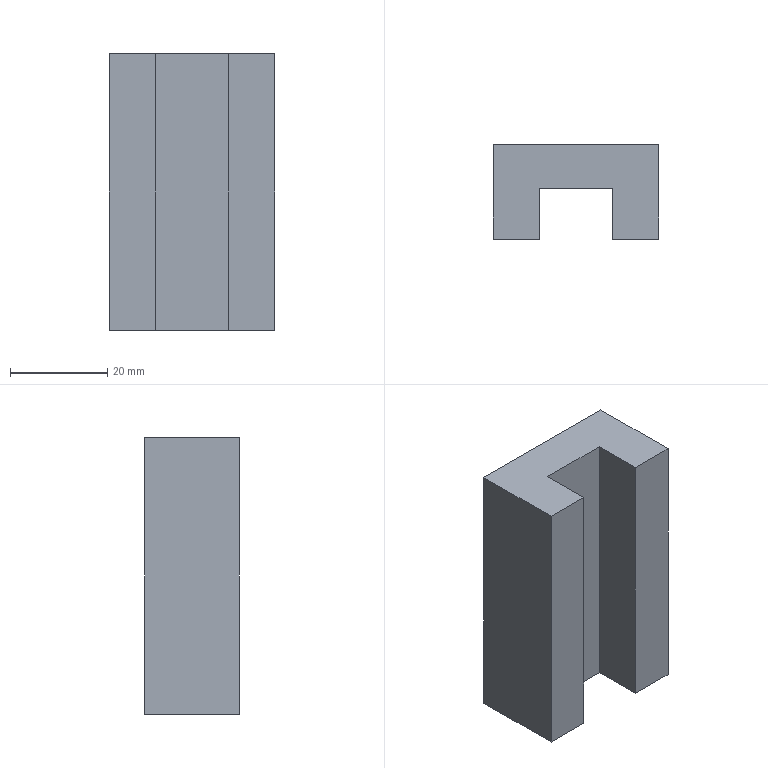Part | SolidWorks | features ICE 2, Extrusion 1 | 1 solid | 22 faces | box 34 x 19.5 x 56.8 mm | volume 28468 mm3 | plane 14 | cylinder 8 | commonest cylinder face diameters 3.6 x8
STEP:
#1=CARTESIAN_POINT('',(-13.,3.75,11.2));
#2=VERTEX_POINT('',#1);
#3=CARTESIAN_POINT('',(-13.,3.75,14.8));
#4=VERTEX_POINT('',#3);
#5=CARTESIAN_POINT('',(-13.,3.75,13.));
#6=DIRECTION('',(0.,1.,0.));
#7=DIRECTION('',(0.,0.,-1.));
#8=AXIS2_PLACEMENT_3D('',#5,#6,#7);
#9=CIRCLE('',#8,1.8);
#10=EDGE_CURVE('',#2,#4,#9,.T.);
#11=ORIENTED_EDGE('',*,*,#10,.F.);
#12=CARTESIAN_POINT('',(-13.,9.75,11.2));
#13=VERTEX_POINT('',#12);
#14=CARTESIAN_POINT('',(-13.,3.75,11.2));
#15=DIRECTION('',(0.,1.,0.));
#16=VECTOR('',#15,1000.);
#17=LINE('',#14,#16);
#18=EDGE_CURVE('',#2,#13,#17,.T.);
#19=ORIENTED_EDGE('',*,*,#18,.T.);
#20=CARTESIAN_POINT('',(-13.,9.75,14.8));
#21=VERTEX_POINT('',#20);
#22=CARTESIAN_POINT('',(-13.,9.75,13.));
#23=DIRECTION('',(0.,1.,0.));
#24=DIRECTION('',(0.,0.,-1.));
#25=AXIS2_PLACEMENT_3D('',#22,#23,#24);
#26=CIRCLE('',#25,1.8);
#27=EDGE_CURVE('',#13,#21,#26,.T.);
#28=ORIENTED_EDGE('',*,*,#27,.T.);
#29=CARTESIAN_POINT('',(-13.,3.75,14.8));
#30=DIRECTION('',(0.,1.,0.));
#31=VECTOR('',#30,1000.);
#32=LINE('',#29,#31);
#33=EDGE_CURVE('',#4,#21,#32,.T.);
#34=ORIENTED_EDGE('',*,*,#33,.F.);
#35=EDGE_LOOP('',(#11,#19,#28,#34));
#36=FACE_OUTER_BOUND('',#35,.T.);
#37=CARTESIAN_POINT('',(-13.,3.75,13.));
#38=DIRECTION('',(0.,1.,0.));
#39=DIRECTION('',(0.,0.,1.));
#40=AXIS2_PLACEMENT_3D('',#37,#38,#39);
#41=CYLINDRICAL_SURFACE('',#40,1.8);
#42=ADVANCED_FACE('',(#36),#41,.F.);
#43=CARTESIAN_POINT('',(13.,3.75,11.2));
#44=VERTEX_POINT('',#43);
#45=CARTESIAN_POINT('',(13.,3.75,14.8));
#46=VERTEX_POINT('',#45);
#47=CARTESIAN_POINT('',(13.,3.75,13.));
#48=DIRECTION('',(0.,1.,0.));
#49=DIRECTION('',(0.,0.,1.));
#50=AXIS2_PLACEMENT_3D('',#47,#48,#49);
#51=CIRCLE('',#50,1.8);
#52=EDGE_CURVE('',#44,#46,#51,.T.);
#53=ORIENTED_EDGE('',*,*,#52,.F.);
#54=CARTESIAN_POINT('',(13.,9.75,11.2));
#55=VERTEX_POINT('',#54);
#56=CARTESIAN_POINT('',(13.,3.75,11.2));
#57=DIRECTION('',(0.,1.,0.));
#58=VECTOR('',#57,1000.);
#59=LINE('',#56,#58);
#60=EDGE_CURVE('',#44,#55,#59,.T.);
#61=ORIENTED_EDGE('',*,*,#60,.T.);
#62=CARTESIAN_POINT('',(13.,9.75,14.8));
#63=VERTEX_POINT('',#62);
#64=CARTESIAN_POINT('',(13.,9.75,13.));
#65=DIRECTION('',(0.,1.,0.));
#66=DIRECTION('',(0.,0.,1.));
#67=AXIS2_PLACEMENT_3D('',#64,#65,#66);
#68=CIRCLE('',#67,1.8);
#69=EDGE_CURVE('',#55,#63,#68,.T.);
#70=ORIENTED_EDGE('',*,*,#69,.T.);
#71=CARTESIAN_POINT('',(13.,3.75,14.8));
#72=DIRECTION('',(0.,1.,0.));
#73=VECTOR('',#72,1000.);
#74=LINE('',#71,#73);
#75=EDGE_CURVE('',#46,#63,#74,.T.);
#76=ORIENTED_EDGE('',*,*,#75,.F.);
#77=EDGE_LOOP('',(#53,#61,#70,#76));
#78=FACE_OUTER_BOUND('',#77,.T.);
#79=CARTESIAN_POINT('',(13.,3.75,13.));
#80=DIRECTION('',(0.,1.,0.));
#81=DIRECTION('',(0.,0.,1.));
#82=AXIS2_PLACEMENT_3D('',#79,#80,#81);
#83=CYLINDRICAL_SURFACE('',#82,1.8);
#84=ADVANCED_FACE('',(#78),#83,.F.);
#85=CARTESIAN_POINT('',(13.,3.75,-14.8));
#86=VERTEX_POINT('',#85);
#87=CARTESIAN_POINT('',(13.,3.75,-11.2));
#88=VERTEX_POINT('',#87);
#89=CARTESIAN_POINT('',(13.,3.75,-13.));
#90=DIRECTION('',(0.,1.,0.));
#91=DIRECTION('',(0.,0.,-1.));
#92=AXIS2_PLACEMENT_3D('',#89,#90,#91);
#93=CIRCLE('',#92,1.8);
#94=EDGE_CURVE('',#86,#88,#93,.T.);
#95=ORIENTED_EDGE('',*,*,#94,.F.);
#96=CARTESIAN_POINT('',(13.,9.75,-14.8));
#97=VERTEX_POINT('',#96);
#98=CARTESIAN_POINT('',(13.,3.75,-14.8));
#99=DIRECTION('',(0.,1.,0.));
#100=VECTOR('',#99,1000.);
#101=LINE('',#98,#100);
#102=EDGE_CURVE('',#86,#97,#101,.T.);
#103=ORIENTED_EDGE('',*,*,#102,.T.);
#104=CARTESIAN_POINT('',(13.,9.75,-11.2));
#105=VERTEX_POINT('',#104);
#106=CARTESIAN_POINT('',(13.,9.75,-13.));
#107=DIRECTION('',(0.,1.,0.));
#108=DIRECTION('',(0.,0.,-1.));
#109=AXIS2_PLACEMENT_3D('',#106,#107,#108);
#110=CIRCLE('',#109,1.8);
#111=EDGE_CURVE('',#97,#105,#110,.T.);
#112=ORIENTED_EDGE('',*,*,#111,.T.);
#113=CARTESIAN_POINT('',(13.,3.75,-11.2));
#114=DIRECTION('',(0.,1.,0.));
#115=VECTOR('',#114,1000.);
#116=LINE('',#113,#115);
#117=EDGE_CURVE('',#88,#105,#116,.T.);
#118=ORIENTED_EDGE('',*,*,#117,.F.);
#119=EDGE_LOOP('',(#95,#103,#112,#118));
#120=FACE_OUTER_BOUND('',#119,.T.);
#121=CARTESIAN_POINT('',(13.,3.75,-13.));
#122=DIRECTION('',(0.,1.,0.));
#123=DIRECTION('',(0.,0.,1.));
#124=AXIS2_PLACEMENT_3D('',#121,#122,#123);
#125=CYLINDRICAL_SURFACE('',#124,1.8);
#126=ADVANCED_FACE('',(#120),#125,.F.);
#127=CARTESIAN_POINT('',(-13.,3.75,-14.8));
#128=VERTEX_POINT('',#127);
#129=CARTESIAN_POINT('',(-13.,3.75,-11.2));
#130=VERTEX_POINT('',#129);
#131=CARTESIAN_POINT('',(-13.,3.75,-13.));
#132=DIRECTION('',(0.,1.,0.));
#133=DIRECTION('',(0.,0.,1.));
#134=AXIS2_PLACEMENT_3D('',#131,#132,#133);
#135=CIRCLE('',#134,1.8);
#136=EDGE_CURVE('',#128,#130,#135,.T.);
#137=ORIENTED_EDGE('',*,*,#136,.F.);
#138=CARTESIAN_POINT('',(-13.,9.75,-14.8));
#139=VERTEX_POINT('',#138);
#140=CARTESIAN_POINT('',(-13.,3.75,-14.8));
#141=DIRECTION('',(0.,1.,0.));
#142=VECTOR('',#141,1000.);
#143=LINE('',#140,#142);
#144=EDGE_CURVE('',#128,#139,#143,.T.);
#145=ORIENTED_EDGE('',*,*,#144,.T.);
#146=CARTESIAN_POINT('',(-13.,9.75,-11.2));
#147=VERTEX_POINT('',#146);
#148=CARTESIAN_POINT('',(-13.,9.75,-13.));
#149=DIRECTION('',(0.,1.,0.));
#150=DIRECTION('',(0.,0.,1.));
#151=AXIS2_PLACEMENT_3D('',#148,#149,#150);
#152=CIRCLE('',#151,1.8);
#153=EDGE_CURVE('',#139,#147,#152,.T.);
#154=ORIENTED_EDGE('',*,*,#153,.T.);
#155=CARTESIAN_POINT('',(-13.,3.75,-11.2));
#156=DIRECTION('',(0.,1.,0.));
#157=VECTOR('',#156,1000.);
#158=LINE('',#155,#157);
#159=EDGE_CURVE('',#130,#147,#158,.T.);
#160=ORIENTED_EDGE('',*,*,#159,.F.);
#161=EDGE_LOOP('',(#137,#145,#154,#160));
#162=FACE_OUTER_BOUND('',#161,.T.);
#163=CARTESIAN_POINT('',(-13.,3.75,-13.));
#164=DIRECTION('',(0.,1.,0.));
#165=DIRECTION('',(0.,0.,1.));
#166=AXIS2_PLACEMENT_3D('',#163,#164,#165);
#167=CYLINDRICAL_SURFACE('',#166,1.8);
#168=ADVANCED_FACE('',(#162),#167,.F.);
#169=CARTESIAN_POINT('',(7.5,-9.75,28.4));
#170=VERTEX_POINT('',#169);
#171=CARTESIAN_POINT('',(17.,-9.75,28.4));
#172=VERTEX_POINT('',#171);
#173=CARTESIAN_POINT('',(-17.,-9.75,28.4));
#174=DIRECTION('',(1.,0.,0.));
#175=VECTOR('',#174,1000.);
#176=LINE('',#173,#175);
#177=EDGE_CURVE('',#170,#172,#176,.T.);
#178=ORIENTED_EDGE('',*,*,#177,.F.);
#179=CARTESIAN_POINT('',(7.5,-9.75,-28.4));
#180=VERTEX_POINT('',#179);
#181=CARTESIAN_POINT('',(7.5,-9.75,-28.4));
#182=DIRECTION('',(0.,0.,1.));
#183=VECTOR('',#182,1000.);
#184=LINE('',#181,#183);
#185=EDGE_CURVE('',#180,#170,#184,.T.);
#186=ORIENTED_EDGE('',*,*,#185,.F.);
#187=CARTESIAN_POINT('',(17.,-9.75,-28.4));
#188=VERTEX_POINT('',#187);
#189=CARTESIAN_POINT('',(-17.,-9.75,-28.4));
#190=DIRECTION('',(1.,0.,0.));
#191=VECTOR('',#190,1000.);
#192=LINE('',#189,#191);
#193=EDGE_CURVE('',#180,#188,#192,.T.);
#194=ORIENTED_EDGE('',*,*,#193,.T.);
#195=CARTESIAN_POINT('',(17.,-9.75,28.4));
#196=DIRECTION('',(0.,0.,-1.));
#197=VECTOR('',#196,1000.);
#198=LINE('',#195,#197);
#199=EDGE_CURVE('',#172,#188,#198,.T.);
#200=ORIENTED_EDGE('',*,*,#199,.F.);
#201=EDGE_LOOP('',(#178,#186,#194,#200));
#202=FACE_OUTER_BOUND('',#201,.T.);
#203=CARTESIAN_POINT('',(-17.,-9.75,28.4));
#204=DIRECTION('',(0.,1.,0.));
#205=DIRECTION('',(0.,0.,1.));
#206=AXIS2_PLACEMENT_3D('',#203,#204,#205);
#207=PLANE('',#206);
#208=ADVANCED_FACE('',(#202),#207,.F.);
#209=CARTESIAN_POINT('',(17.,9.75,-28.4));
#210=VERTEX_POINT('',#209);
#211=CARTESIAN_POINT('',(17.,9.75,-28.4));
#212=DIRECTION('',(0.,1.,0.));
#213=VECTOR('',#212,1000.);
#214=LINE('',#211,#213);
#215=EDGE_CURVE('',#188,#210,#214,.T.);
#216=ORIENTED_EDGE('',*,*,#215,.T.);
#217=CARTESIAN_POINT('',(17.,9.75,28.4));
#218=VERTEX_POINT('',#217);
#219=CARTESIAN_POINT('',(17.,9.75,28.4));
#220=DIRECTION('',(0.,0.,-1.));
#221=VECTOR('',#220,1000.);
#222=LINE('',#219,#221);
#223=EDGE_CURVE('',#218,#210,#222,.T.);
#224=ORIENTED_EDGE('',*,*,#223,.F.);
#225=CARTESIAN_POINT('',(17.,9.75,28.4));
#226=DIRECTION('',(0.,1.,0.));
#227=VECTOR('',#226,1000.);
#228=LINE('',#225,#227);
#229=EDGE_CURVE('',#172,#218,#228,.T.);
#230=ORIENTED_EDGE('',*,*,#229,.F.);
#231=ORIENTED_EDGE('',*,*,#199,.T.);
#232=EDGE_LOOP('',(#216,#224,#230,#231));
#233=FACE_OUTER_BOUND('',#232,.T.);
#234=CARTESIAN_POINT('',(17.,9.75,28.4));
#235=DIRECTION('',(-1.,0.,0.));
#236=DIRECTION('',(0.,-1.,0.));
#237=AXIS2_PLACEMENT_3D('',#234,#235,#236);
#238=PLANE('',#237);
#239=ADVANCED_FACE('',(#233),#238,.F.);
#240=CARTESIAN_POINT('',(-13.,9.75,13.));
#241=DIRECTION('',(0.,1.,0.));
#242=DIRECTION('',(0.,0.,-1.));
#243=AXIS2_PLACEMENT_3D('',#240,#241,#242);
#244=CIRCLE('',#243,1.8);
#245=EDGE_CURVE('',#21,#13,#244,.T.);
#246=ORIENTED_EDGE('',*,*,#245,.F.);
#247=ORIENTED_EDGE('',*,*,#27,.F.);
#248=EDGE_LOOP('',(#246,#247));
#249=FACE_BOUND('',#248,.T.);
#250=CARTESIAN_POINT('',(13.,9.75,13.));
#251=DIRECTION('',(0.,1.,0.));
#252=DIRECTION('',(0.,0.,1.));
#253=AXIS2_PLACEMENT_3D('',#250,#251,#252);
#254=CIRCLE('',#253,1.8);
#255=EDGE_CURVE('',#63,#55,#254,.T.);
#256=ORIENTED_EDGE('',*,*,#255,.F.);
#257=ORIENTED_EDGE('',*,*,#69,.F.);
#258=EDGE_LOOP('',(#256,#257));
#259=FACE_BOUND('',#258,.T.);
#260=CARTESIAN_POINT('',(13.,9.75,-13.));
#261=DIRECTION('',(0.,1.,0.));
#262=DIRECTION('',(0.,0.,-1.));
#263=AXIS2_PLACEMENT_3D('',#260,#261,#262);
#264=CIRCLE('',#263,1.8);
#265=EDGE_CURVE('',#105,#97,#264,.T.);
#266=ORIENTED_EDGE('',*,*,#265,.F.);
#267=ORIENTED_EDGE('',*,*,#111,.F.);
#268=EDGE_LOOP('',(#266,#267));
#269=FACE_BOUND('',#268,.T.);
#270=CARTESIAN_POINT('',(-13.,9.75,-13.));
#271=DIRECTION('',(0.,1.,0.));
#272=DIRECTION('',(0.,0.,1.));
#273=AXIS2_PLACEMENT_3D('',#270,#271,#272);
#274=CIRCLE('',#273,1.8);
#275=EDGE_CURVE('',#147,#139,#274,.T.);
#276=ORIENTED_EDGE('',*,*,#275,.F.);
#277=ORIENTED_EDGE('',*,*,#153,.F.);
#278=EDGE_LOOP('',(#276,#277));
#279=FACE_BOUND('',#278,.T.);
#280=CARTESIAN_POINT('',(-17.,9.75,-28.4));
#281=VERTEX_POINT('',#280);
#282=CARTESIAN_POINT('',(-17.,9.75,-28.4));
#283=DIRECTION('',(-1.,0.,0.));
#284=VECTOR('',#283,1000.);
#285=LINE('',#282,#284);
#286=EDGE_CURVE('',#210,#281,#285,.T.);
#287=ORIENTED_EDGE('',*,*,#286,.T.);
#288=CARTESIAN_POINT('',(-17.,9.75,28.4));
#289=VERTEX_POINT('',#288);
#290=CARTESIAN_POINT('',(-17.,9.75,28.4));
#291=DIRECTION('',(0.,0.,-1.));
#292=VECTOR('',#291,1000.);
#293=LINE('',#290,#292);
#294=EDGE_CURVE('',#289,#281,#293,.T.);
#295=ORIENTED_EDGE('',*,*,#294,.F.);
#296=CARTESIAN_POINT('',(-17.,9.75,28.4));
#297=DIRECTION('',(-1.,0.,0.));
#298=VECTOR('',#297,1000.);
#299=LINE('',#296,#298);
#300=EDGE_CURVE('',#218,#289,#299,.T.);
#301=ORIENTED_EDGE('',*,*,#300,.F.);
#302=ORIENTED_EDGE('',*,*,#223,.T.);
#303=EDGE_LOOP('',(#287,#295,#301,#302));
#304=FACE_OUTER_BOUND('',#303,.T.);
#305=CARTESIAN_POINT('',(-17.,9.75,28.4));
#306=DIRECTION('',(0.,-1.,0.));
#307=DIRECTION('',(0.,0.,-1.));
#308=AXIS2_PLACEMENT_3D('',#305,#306,#307);
#309=PLANE('',#308);
#310=ADVANCED_FACE('',(#249,#259,#269,#279,#304),#309,.F.);
#311=CARTESIAN_POINT('',(-17.,-9.75,-28.4));
#312=VERTEX_POINT('',#311);
#313=CARTESIAN_POINT('',(-17.,9.75,-28.4));
#314=DIRECTION('',(0.,-1.,0.));
#315=VECTOR('',#314,1000.);
#316=LINE('',#313,#315);
#317=EDGE_CURVE('',#281,#312,#316,.T.);
#318=ORIENTED_EDGE('',*,*,#317,.T.);
#319=CARTESIAN_POINT('',(-17.,-9.75,28.4));
#320=VERTEX_POINT('',#319);
#321=CARTESIAN_POINT('',(-17.,-9.75,28.4));
#322=DIRECTION('',(0.,0.,-1.));
#323=VECTOR('',#322,1000.);
#324=LINE('',#321,#323);
#325=EDGE_CURVE('',#320,#312,#324,.T.);
#326=ORIENTED_EDGE('',*,*,#325,.F.);
#327=CARTESIAN_POINT('',(-17.,9.75,28.4));
#328=DIRECTION('',(0.,-1.,0.));
#329=VECTOR('',#328,1000.);
#330=LINE('',#327,#329);
#331=EDGE_CURVE('',#289,#320,#330,.T.);
#332=ORIENTED_EDGE('',*,*,#331,.F.);
#333=ORIENTED_EDGE('',*,*,#294,.T.);
#334=EDGE_LOOP('',(#318,#326,#332,#333));
#335=FACE_OUTER_BOUND('',#334,.T.);
#336=CARTESIAN_POINT('',(-17.,9.75,28.4));
#337=DIRECTION('',(1.,0.,0.));
#338=DIRECTION('',(0.,1.,0.));
#339=AXIS2_PLACEMENT_3D('',#336,#337,#338);
#340=PLANE('',#339);
#341=ADVANCED_FACE('',(#335),#340,.F.);
#342=CARTESIAN_POINT('',(-7.5,-9.75,-28.4));
#343=VERTEX_POINT('',#342);
#344=CARTESIAN_POINT('',(-17.,-9.75,-28.4));
#345=DIRECTION('',(1.,0.,0.));
#346=VECTOR('',#345,1000.);
#347=LINE('',#344,#346);
#348=EDGE_CURVE('',#312,#343,#347,.T.);
#349=ORIENTED_EDGE('',*,*,#348,.T.);
#350=CARTESIAN_POINT('',(-7.5,-9.75,28.4));
#351=VERTEX_POINT('',#350);
#352=CARTESIAN_POINT('',(-7.5,-9.75,-28.4));
#353=DIRECTION('',(0.,0.,1.));
#354=VECTOR('',#353,1000.);
#355=LINE('',#352,#354);
#356=EDGE_CURVE('',#343,#351,#355,.T.);
#357=ORIENTED_EDGE('',*,*,#356,.T.);
#358=CARTESIAN_POINT('',(-17.,-9.75,28.4));
#359=DIRECTION('',(1.,0.,0.));
#360=VECTOR('',#359,1000.);
#361=LINE('',#358,#360);
#362=EDGE_CURVE('',#320,#351,#361,.T.);
#363=ORIENTED_EDGE('',*,*,#362,.F.);
#364=ORIENTED_EDGE('',*,*,#325,.T.);
#365=EDGE_LOOP('',(#349,#357,#363,#364));
#366=FACE_OUTER_BOUND('',#365,.T.);
#367=CARTESIAN_POINT('',(-17.,-9.75,28.4));
#368=DIRECTION('',(0.,1.,0.));
#369=DIRECTION('',(0.,0.,1.));
#370=AXIS2_PLACEMENT_3D('',#367,#368,#369);
#371=PLANE('',#370);
#372=ADVANCED_FACE('',(#366),#371,.F.);
#373=CARTESIAN_POINT('',(7.5,0.75,28.4));
#374=VERTEX_POINT('',#373);
#375=CARTESIAN_POINT('',(7.5,0.75,28.4));
#376=DIRECTION('',(0.,1.,0.));
#377=VECTOR('',#376,1000.);
#378=LINE('',#375,#377);
#379=EDGE_CURVE('',#170,#374,#378,.T.);
#380=ORIENTED_EDGE('',*,*,#379,.F.);
#381=ORIENTED_EDGE('',*,*,#177,.T.);
#382=ORIENTED_EDGE('',*,*,#229,.T.);
#383=ORIENTED_EDGE('',*,*,#300,.T.);
#384=ORIENTED_EDGE('',*,*,#331,.T.);
#385=ORIENTED_EDGE('',*,*,#362,.T.);
#386=CARTESIAN_POINT('',(-7.5,0.75,28.4));
#387=VERTEX_POINT('',#386);
#388=CARTESIAN_POINT('',(-7.5,0.75,28.4));
#389=DIRECTION('',(0.,-1.,0.));
#390=VECTOR('',#389,1000.);
#391=LINE('',#388,#390);
#392=EDGE_CURVE('',#387,#351,#391,.T.);
#393=ORIENTED_EDGE('',*,*,#392,.F.);
#394=CARTESIAN_POINT('',(-7.5,0.75,28.4));
#395=DIRECTION('',(-1.,0.,0.));
#396=VECTOR('',#395,1000.);
#397=LINE('',#394,#396);
#398=EDGE_CURVE('',#374,#387,#397,.T.);
#399=ORIENTED_EDGE('',*,*,#398,.F.);
#400=EDGE_LOOP('',(#380,#381,#382,#383,#384,#385,#393,#399));
#401=FACE_OUTER_BOUND('',#400,.T.);
#402=CARTESIAN_POINT('',(0.,0.,28.4));
#403=DIRECTION('',(0.,0.,1.));
#404=DIRECTION('',(1.,0.,0.));
#405=AXIS2_PLACEMENT_3D('',#402,#403,#404);
#406=PLANE('',#405);
#407=ADVANCED_FACE('',(#401),#406,.T.);
#408=ORIENTED_EDGE('',*,*,#193,.F.);
#409=CARTESIAN_POINT('',(7.5,0.75,-28.4));
#410=VERTEX_POINT('',#409);
#411=CARTESIAN_POINT('',(7.5,0.75,-28.4));
#412=DIRECTION('',(0.,1.,0.));
#413=VECTOR('',#412,1000.);
#414=LINE('',#411,#413);
#415=EDGE_CURVE('',#180,#410,#414,.T.);
#416=ORIENTED_EDGE('',*,*,#415,.T.);
#417=CARTESIAN_POINT('',(-7.5,0.75,-28.4));
#418=VERTEX_POINT('',#417);
#419=CARTESIAN_POINT('',(-7.5,0.75,-28.4));
#420=DIRECTION('',(-1.,0.,0.));
#421=VECTOR('',#420,1000.);
#422=LINE('',#419,#421);
#423=EDGE_CURVE('',#410,#418,#422,.T.);
#424=ORIENTED_EDGE('',*,*,#423,.T.);
#425=CARTESIAN_POINT('',(-7.5,0.75,-28.4));
#426=DIRECTION('',(0.,-1.,0.));
#427=VECTOR('',#426,1000.);
#428=LINE('',#425,#427);
#429=EDGE_CURVE('',#418,#343,#428,.T.);
#430=ORIENTED_EDGE('',*,*,#429,.T.);
#431=ORIENTED_EDGE('',*,*,#348,.F.);
#432=ORIENTED_EDGE('',*,*,#317,.F.);
#433=ORIENTED_EDGE('',*,*,#286,.F.);
#434=ORIENTED_EDGE('',*,*,#215,.F.);
#435=EDGE_LOOP('',(#408,#416,#424,#430,#431,#432,#433,#434));
#436=FACE_OUTER_BOUND('',#435,.T.);
#437=CARTESIAN_POINT('',(0.,0.,-28.4));
#438=DIRECTION('',(0.,0.,1.));
#439=DIRECTION('',(1.,0.,0.));
#440=AXIS2_PLACEMENT_3D('',#437,#438,#439);
#441=PLANE('',#440);
#442=ADVANCED_FACE('',(#436),#441,.F.);
#443=CARTESIAN_POINT('',(7.5,0.75,-28.4));
#444=DIRECTION('',(0.,0.,1.));
#445=VECTOR('',#444,1000.);
#446=LINE('',#443,#445);
#447=EDGE_CURVE('',#410,#374,#446,.T.);
#448=ORIENTED_EDGE('',*,*,#447,.F.);
#449=ORIENTED_EDGE('',*,*,#415,.F.);
#450=ORIENTED_EDGE('',*,*,#185,.T.);
#451=ORIENTED_EDGE('',*,*,#379,.T.);
#452=EDGE_LOOP('',(#448,#449,#450,#451));
#453=FACE_OUTER_BOUND('',#452,.T.);
#454=CARTESIAN_POINT('',(7.5,0.75,-28.4));
#455=DIRECTION('',(1.,0.,0.));
#456=DIRECTION('',(0.,1.,0.));
#457=AXIS2_PLACEMENT_3D('',#454,#455,#456);
#458=PLANE('',#457);
#459=ADVANCED_FACE('',(#453),#458,.F.);
#460=ORIENTED_EDGE('',*,*,#356,.F.);
#461=ORIENTED_EDGE('',*,*,#429,.F.);
#462=CARTESIAN_POINT('',(-7.5,0.75,-28.4));
#463=DIRECTION('',(0.,0.,1.));
#464=VECTOR('',#463,1000.);
#465=LINE('',#462,#464);
#466=EDGE_CURVE('',#418,#387,#465,.T.);
#467=ORIENTED_EDGE('',*,*,#466,.T.);
#468=ORIENTED_EDGE('',*,*,#392,.T.);
#469=EDGE_LOOP('',(#460,#461,#467,#468));
#470=FACE_OUTER_BOUND('',#469,.T.);
#471=CARTESIAN_POINT('',(-7.5,0.75,-28.4));
#472=DIRECTION('',(-1.,0.,0.));
#473=DIRECTION('',(0.,-1.,0.));
#474=AXIS2_PLACEMENT_3D('',#471,#472,#473);
#475=PLANE('',#474);
#476=ADVANCED_FACE('',(#470),#475,.F.);
#477=ORIENTED_EDGE('',*,*,#466,.F.);
#478=ORIENTED_EDGE('',*,*,#423,.F.);
#479=ORIENTED_EDGE('',*,*,#447,.T.);
#480=ORIENTED_EDGE('',*,*,#398,.T.);
#481=EDGE_LOOP('',(#477,#478,#479,#480));
#482=FACE_OUTER_BOUND('',#481,.T.);
#483=CARTESIAN_POINT('',(-7.5,0.75,-28.4));
#484=DIRECTION('',(0.,1.,0.));
#485=DIRECTION('',(0.,0.,1.));
#486=AXIS2_PLACEMENT_3D('',#483,#484,#485);
#487=PLANE('',#486);
#488=ADVANCED_FACE('',(#482),#487,.F.);
#489=ORIENTED_EDGE('',*,*,#144,.F.);
#490=CARTESIAN_POINT('',(-13.,3.75,-13.));
#491=DIRECTION('',(0.,1.,0.));
#492=DIRECTION('',(0.,0.,1.));
#493=AXIS2_PLACEMENT_3D('',#490,#491,#492);
#494=CIRCLE('',#493,1.8);
#495=EDGE_CURVE('',#130,#128,#494,.T.);
#496=ORIENTED_EDGE('',*,*,#495,.F.);
#497=ORIENTED_EDGE('',*,*,#159,.T.);
#498=ORIENTED_EDGE('',*,*,#275,.T.);
#499=EDGE_LOOP('',(#489,#496,#497,#498));
#500=FACE_OUTER_BOUND('',#499,.T.);
#501=CARTESIAN_POINT('',(-13.,3.75,-13.));
#502=DIRECTION('',(0.,1.,0.));
#503=DIRECTION('',(0.,0.,1.));
#504=AXIS2_PLACEMENT_3D('',#501,#502,#503);
#505=CYLINDRICAL_SURFACE('',#504,1.8);
#506=ADVANCED_FACE('',(#500),#505,.F.);
#507=ORIENTED_EDGE('',*,*,#495,.T.);
#508=ORIENTED_EDGE('',*,*,#136,.T.);
#509=EDGE_LOOP('',(#507,#508));
#510=FACE_OUTER_BOUND('',#509,.T.);
#511=CARTESIAN_POINT('',(-13.,3.75,-13.));
#512=DIRECTION('',(0.,1.,0.));
#513=DIRECTION('',(0.,0.,1.));
#514=AXIS2_PLACEMENT_3D('',#511,#512,#513);
#515=PLANE('',#514);
#516=ADVANCED_FACE('',(#510),#515,.T.);
#517=ORIENTED_EDGE('',*,*,#102,.F.);
#518=CARTESIAN_POINT('',(13.,3.75,-13.));
#519=DIRECTION('',(0.,1.,0.));
#520=DIRECTION('',(0.,0.,-1.));
#521=AXIS2_PLACEMENT_3D('',#518,#519,#520);
#522=CIRCLE('',#521,1.8);
#523=EDGE_CURVE('',#88,#86,#522,.T.);
#524=ORIENTED_EDGE('',*,*,#523,.F.);
#525=ORIENTED_EDGE('',*,*,#117,.T.);
#526=ORIENTED_EDGE('',*,*,#265,.T.);
#527=EDGE_LOOP('',(#517,#524,#525,#526));
#528=FACE_OUTER_BOUND('',#527,.T.);
#529=CARTESIAN_POINT('',(13.,3.75,-13.));
#530=DIRECTION('',(0.,1.,0.));
#531=DIRECTION('',(0.,0.,1.));
#532=AXIS2_PLACEMENT_3D('',#529,#530,#531);
#533=CYLINDRICAL_SURFACE('',#532,1.8);
#534=ADVANCED_FACE('',(#528),#533,.F.);
#535=ORIENTED_EDGE('',*,*,#523,.T.);
#536=ORIENTED_EDGE('',*,*,#94,.T.);
#537=EDGE_LOOP('',(#535,#536));
#538=FACE_OUTER_BOUND('',#537,.T.);
#539=CARTESIAN_POINT('',(13.,3.75,-13.));
#540=DIRECTION('',(0.,-1.,0.));
#541=DIRECTION('',(0.,0.,-1.));
#542=AXIS2_PLACEMENT_3D('',#539,#540,#541);
#543=PLANE('',#542);
#544=ADVANCED_FACE('',(#538),#543,.F.);
#545=ORIENTED_EDGE('',*,*,#60,.F.);
#546=CARTESIAN_POINT('',(13.,3.75,13.));
#547=DIRECTION('',(0.,1.,0.));
#548=DIRECTION('',(0.,0.,1.));
#549=AXIS2_PLACEMENT_3D('',#546,#547,#548);
#550=CIRCLE('',#549,1.8);
#551=EDGE_CURVE('',#46,#44,#550,.T.);
#552=ORIENTED_EDGE('',*,*,#551,.F.);
#553=ORIENTED_EDGE('',*,*,#75,.T.);
#554=ORIENTED_EDGE('',*,*,#255,.T.);
#555=EDGE_LOOP('',(#545,#552,#553,#554));
#556=FACE_OUTER_BOUND('',#555,.T.);
#557=CARTESIAN_POINT('',(13.,3.75,13.));
#558=DIRECTION('',(0.,1.,0.));
#559=DIRECTION('',(0.,0.,1.));
#560=AXIS2_PLACEMENT_3D('',#557,#558,#559);
#561=CYLINDRICAL_SURFACE('',#560,1.8);
#562=ADVANCED_FACE('',(#556),#561,.F.);
#563=ORIENTED_EDGE('',*,*,#551,.T.);
#564=ORIENTED_EDGE('',*,*,#52,.T.);
#565=EDGE_LOOP('',(#563,#564));
#566=FACE_OUTER_BOUND('',#565,.T.);
#567=CARTESIAN_POINT('',(13.,3.75,13.));
#568=DIRECTION('',(0.,1.,0.));
#569=DIRECTION('',(0.,0.,1.));
#570=AXIS2_PLACEMENT_3D('',#567,#568,#569);
#571=PLANE('',#570);
#572=ADVANCED_FACE('',(#566),#571,.T.);
#573=ORIENTED_EDGE('',*,*,#18,.F.);
#574=CARTESIAN_POINT('',(-13.,3.75,13.));
#575=DIRECTION('',(0.,1.,0.));
#576=DIRECTION('',(0.,0.,-1.));
#577=AXIS2_PLACEMENT_3D('',#574,#575,#576);
#578=CIRCLE('',#577,1.8);
#579=EDGE_CURVE('',#4,#2,#578,.T.);
#580=ORIENTED_EDGE('',*,*,#579,.F.);
#581=ORIENTED_EDGE('',*,*,#33,.T.);
#582=ORIENTED_EDGE('',*,*,#245,.T.);
#583=EDGE_LOOP('',(#573,#580,#581,#582));
#584=FACE_OUTER_BOUND('',#583,.T.);
#585=CARTESIAN_POINT('',(-13.,3.75,13.));
#586=DIRECTION('',(0.,1.,0.));
#587=DIRECTION('',(0.,0.,1.));
#588=AXIS2_PLACEMENT_3D('',#585,#586,#587);
#589=CYLINDRICAL_SURFACE('',#588,1.8);
#590=ADVANCED_FACE('',(#584),#589,.F.);
#591=ORIENTED_EDGE('',*,*,#579,.T.);
#592=ORIENTED_EDGE('',*,*,#10,.T.);
#593=EDGE_LOOP('',(#591,#592));
#594=FACE_OUTER_BOUND('',#593,.T.);
#595=CARTESIAN_POINT('',(-13.,3.75,13.));
#596=DIRECTION('',(0.,-1.,0.));
#597=DIRECTION('',(0.,0.,-1.));
#598=AXIS2_PLACEMENT_3D('',#595,#596,#597);
#599=PLANE('',#598);
#600=ADVANCED_FACE('',(#594),#599,.F.);
#601=CLOSED_SHELL('',(#42,#84,#126,#168,#208,#239,#310,#341,#372,#407,#442,#459,#476,#488,#506,#516,#534,#544,#562,#572,#590,#600));
#602=MANIFOLD_SOLID_BREP('',#601);
#603=CARTESIAN_POINT('',(0.,0.,0.));
#604=DIRECTION('',(0.,0.,1.));
#605=DIRECTION('',(1.,0.,0.));
#606=AXIS2_PLACEMENT_3D('',#603,#604,#605);
#607=(LENGTH_UNIT()NAMED_UNIT(*)SI_UNIT(.MILLI.,.METRE.));
#608=UNCERTAINTY_MEASURE_WITH_UNIT(LENGTH_MEASURE(0.00001),#607,'','');
#609=(NAMED_UNIT(*)PLANE_ANGLE_UNIT()SI_UNIT($,.RADIAN.));
#610=(NAMED_UNIT(*)SI_UNIT($,.STERADIAN.)SOLID_ANGLE_UNIT());
#611=(GEOMETRIC_REPRESENTATION_CONTEXT(3)GLOBAL_UNCERTAINTY_ASSIGNED_CONTEXT((#608))GLOBAL_UNIT_ASSIGNED_CONTEXT((#607,#609,#610))REPRESENTATION_CONTEXT('',''));
#612=ADVANCED_BREP_SHAPE_REPRESENTATION('',(#602,#606),#611);